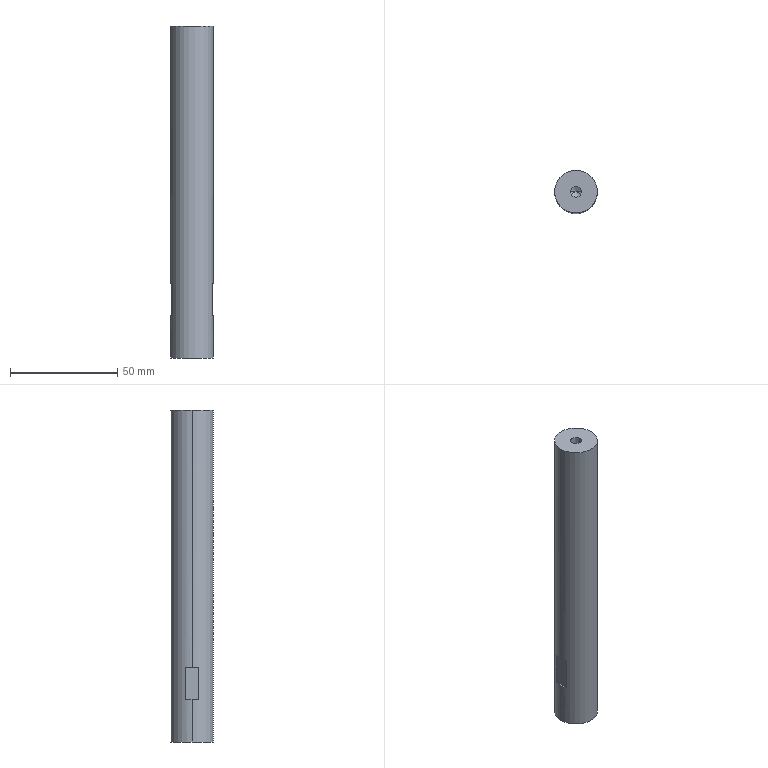Part | STEP file | slingshot displacement cylinder seat post | 1 solid | 18 faces | box 20 x 20 x 155 mm | volume 47945 mm3 | plane 8 | cylinder 6 | cone 4 | commonest cylinder face diameters 5 x4 20 x2
STEP:
#1=CARTESIAN_POINT('',(0.,0.,0.));
#2=DIRECTION('',(0.,0.,1.));
#3=DIRECTION('',(1.,0.,0.));
#4=AXIS2_PLACEMENT_3D('',#1,#2,#3);
#5=CARTESIAN_POINT('',(-2.5,0.,138.));
#6=VERTEX_POINT('',#5);
#7=CARTESIAN_POINT('',(2.5,0.,138.));
#8=VERTEX_POINT('',#7);
#9=CARTESIAN_POINT('',(0.,0.,138.));
#10=DIRECTION('',(0.,0.,1.));
#11=DIRECTION('',(1.,0.,0.));
#12=AXIS2_PLACEMENT_3D('',#9,#10,#11);
#13=CIRCLE('',#12,2.5);
#14=CARTESIAN_POINT('',(0.,0.,138.));
#15=DIRECTION('',(0.,0.,1.));
#16=DIRECTION('',(1.,0.,0.));
#17=AXIS2_PLACEMENT_3D('',#14,#15,#16);
#18=CONICAL_SURFACE('',#17,2.5,1.03);
#19=CARTESIAN_POINT('',(0.,0.));
#20=DIRECTION('',(1.,0.));
#21=VECTOR('',#20,1.);
#22=LINE('',#19,#21);
#23=(GEOMETRIC_REPRESENTATION_CONTEXT(2)PARAMETRIC_REPRESENTATION_CONTEXT()REPRESENTATION_CONTEXT('',''));
#24=DEFINITIONAL_REPRESENTATION('',(#22),#23);
#25=PCURVE('',#18,#24);
#26=CARTESIAN_POINT('',(0.,0.,155.));
#27=DIRECTION('',(0.,0.,1.));
#28=DIRECTION('',(1.,0.,0.));
#29=AXIS2_PLACEMENT_3D('',#26,#27,#28);
#30=CYLINDRICAL_SURFACE('',#29,2.5);
#31=CARTESIAN_POINT('',(0.,-17.));
#32=DIRECTION('',(1.,0.));
#33=VECTOR('',#32,1.);
#34=LINE('',#31,#33);
#35=(GEOMETRIC_REPRESENTATION_CONTEXT(2)PARAMETRIC_REPRESENTATION_CONTEXT()REPRESENTATION_CONTEXT('',''));
#36=DEFINITIONAL_REPRESENTATION('',(#34),#35);
#37=PCURVE('',#30,#36);
#38=SURFACE_CURVE('',#13,(#25,#37),.PCURVE_S1.);
#39=EDGE_CURVE('',#6,#8,#38,.T.);
#40=ORIENTED_EDGE('',*,*,#39,.F.);
#41=CARTESIAN_POINT('',(0.,0.,136.498));
#42=VERTEX_POINT('',#41);
#43=CARTESIAN_POINT('',(-2.5,0.,138.));
#44=DIRECTION('',(-0.8572,0.,0.515));
#45=VECTOR('',#44,1.);
#46=LINE('',#43,#45);
#47=CARTESIAN_POINT('',(3.142,0.));
#48=DIRECTION('',(0.,1.));
#49=VECTOR('',#48,1.);
#50=LINE('',#47,#49);
#51=(GEOMETRIC_REPRESENTATION_CONTEXT(2)PARAMETRIC_REPRESENTATION_CONTEXT()REPRESENTATION_CONTEXT('',''));
#52=DEFINITIONAL_REPRESENTATION('',(#50),#51);
#53=PCURVE('',#18,#52);
#54=CARTESIAN_POINT('',(0.,0.,138.));
#55=DIRECTION('',(0.,0.,1.));
#56=DIRECTION('',(1.,0.,0.));
#57=AXIS2_PLACEMENT_3D('',#54,#55,#56);
#58=CONICAL_SURFACE('',#57,2.5,1.03);
#59=CARTESIAN_POINT('',(3.142,0.));
#60=DIRECTION('',(0.,1.));
#61=VECTOR('',#60,1.);
#62=LINE('',#59,#61);
#63=(GEOMETRIC_REPRESENTATION_CONTEXT(2)PARAMETRIC_REPRESENTATION_CONTEXT()REPRESENTATION_CONTEXT('',''));
#64=DEFINITIONAL_REPRESENTATION('',(#62),#63);
#65=PCURVE('',#58,#64);
#66=SURFACE_CURVE('',#46,(#53,#65),.PCURVE_S1.);
#67=EDGE_CURVE('',#42,#6,#66,.T.);
#68=ORIENTED_EDGE('',*,*,#67,.F.);
#69=CARTESIAN_POINT('',(2.5,0.,138.));
#70=DIRECTION('',(0.8572,0.,0.515));
#71=VECTOR('',#70,1.);
#72=LINE('',#69,#71);
#73=CARTESIAN_POINT('',(6.283,0.));
#74=DIRECTION('',(0.,1.));
#75=VECTOR('',#74,1.);
#76=LINE('',#73,#75);
#77=(GEOMETRIC_REPRESENTATION_CONTEXT(2)PARAMETRIC_REPRESENTATION_CONTEXT()REPRESENTATION_CONTEXT('',''));
#78=DEFINITIONAL_REPRESENTATION('',(#76),#77);
#79=PCURVE('',#18,#78);
#80=CARTESIAN_POINT('',(0.,0.));
#81=DIRECTION('',(0.,1.));
#82=VECTOR('',#81,1.);
#83=LINE('',#80,#82);
#84=(GEOMETRIC_REPRESENTATION_CONTEXT(2)PARAMETRIC_REPRESENTATION_CONTEXT()REPRESENTATION_CONTEXT('',''));
#85=DEFINITIONAL_REPRESENTATION('',(#83),#84);
#86=PCURVE('',#58,#85);
#87=SURFACE_CURVE('',#72,(#79,#86),.PCURVE_S1.);
#88=EDGE_CURVE('',#42,#8,#87,.T.);
#89=ORIENTED_EDGE('',*,*,#88,.T.);
#90=EDGE_LOOP('',(#40,#68,#89));
#91=FACE_BOUND('',#90,.F.);
#92=ADVANCED_FACE('',(#91),#18,.F.);
#93=CARTESIAN_POINT('',(2.5,0.,155.));
#94=VERTEX_POINT('',#93);
#95=CARTESIAN_POINT('',(2.5,0.,155.));
#96=DIRECTION('',(0.,0.,1.));
#97=VECTOR('',#96,1.);
#98=LINE('',#95,#97);
#99=CARTESIAN_POINT('',(6.283,0.));
#100=DIRECTION('',(0.,1.));
#101=VECTOR('',#100,1.);
#102=LINE('',#99,#101);
#103=(GEOMETRIC_REPRESENTATION_CONTEXT(2)PARAMETRIC_REPRESENTATION_CONTEXT()REPRESENTATION_CONTEXT('',''));
#104=DEFINITIONAL_REPRESENTATION('',(#102),#103);
#105=PCURVE('',#30,#104);
#106=CARTESIAN_POINT('',(0.,0.,155.));
#107=DIRECTION('',(0.,0.,1.));
#108=DIRECTION('',(1.,0.,0.));
#109=AXIS2_PLACEMENT_3D('',#106,#107,#108);
#110=CYLINDRICAL_SURFACE('',#109,2.5);
#111=CARTESIAN_POINT('',(0.,0.));
#112=DIRECTION('',(0.,1.));
#113=VECTOR('',#112,1.);
#114=LINE('',#111,#113);
#115=(GEOMETRIC_REPRESENTATION_CONTEXT(2)PARAMETRIC_REPRESENTATION_CONTEXT()REPRESENTATION_CONTEXT('',''));
#116=DEFINITIONAL_REPRESENTATION('',(#114),#115);
#117=PCURVE('',#110,#116);
#118=SURFACE_CURVE('',#98,(#105,#117),.PCURVE_S1.);
#119=EDGE_CURVE('',#8,#94,#118,.T.);
#120=ORIENTED_EDGE('',*,*,#119,.T.);
#121=CARTESIAN_POINT('',(-2.5,0.,155.));
#122=VERTEX_POINT('',#121);
#123=CARTESIAN_POINT('',(0.,0.,155.));
#124=DIRECTION('',(0.,0.,1.));
#125=DIRECTION('',(1.,0.,0.));
#126=AXIS2_PLACEMENT_3D('',#123,#124,#125);
#127=CIRCLE('',#126,2.5);
#128=CARTESIAN_POINT('',(0.,0.));
#129=DIRECTION('',(1.,0.));
#130=VECTOR('',#129,1.);
#131=LINE('',#128,#130);
#132=(GEOMETRIC_REPRESENTATION_CONTEXT(2)PARAMETRIC_REPRESENTATION_CONTEXT()REPRESENTATION_CONTEXT('',''));
#133=DEFINITIONAL_REPRESENTATION('',(#131),#132);
#134=PCURVE('',#30,#133);
#135=CARTESIAN_POINT('',(0.,0.,155.));
#136=DIRECTION('',(0.,0.,1.));
#137=DIRECTION('',(1.,0.,0.));
#138=AXIS2_PLACEMENT_3D('',#135,#136,#137);
#139=PLANE('',#138);
#140=CARTESIAN_POINT('',(0.,0.));
#141=DIRECTION('',(1.,0.));
#142=AXIS2_PLACEMENT_2D('',#140,#141);
#143=CIRCLE('',#142,2.5);
#144=(GEOMETRIC_REPRESENTATION_CONTEXT(2)PARAMETRIC_REPRESENTATION_CONTEXT()REPRESENTATION_CONTEXT('',''));
#145=DEFINITIONAL_REPRESENTATION('',(#143),#144);
#146=PCURVE('',#139,#145);
#147=SURFACE_CURVE('',#127,(#134,#146),.PCURVE_S1.);
#148=EDGE_CURVE('',#122,#94,#147,.T.);
#149=ORIENTED_EDGE('',*,*,#148,.F.);
#150=CARTESIAN_POINT('',(-2.5,0.,155.));
#151=DIRECTION('',(0.,0.,1.));
#152=VECTOR('',#151,1.);
#153=LINE('',#150,#152);
#154=CARTESIAN_POINT('',(3.142,0.));
#155=DIRECTION('',(0.,1.));
#156=VECTOR('',#155,1.);
#157=LINE('',#154,#156);
#158=(GEOMETRIC_REPRESENTATION_CONTEXT(2)PARAMETRIC_REPRESENTATION_CONTEXT()REPRESENTATION_CONTEXT('',''));
#159=DEFINITIONAL_REPRESENTATION('',(#157),#158);
#160=PCURVE('',#30,#159);
#161=CARTESIAN_POINT('',(3.142,0.));
#162=DIRECTION('',(0.,1.));
#163=VECTOR('',#162,1.);
#164=LINE('',#161,#163);
#165=(GEOMETRIC_REPRESENTATION_CONTEXT(2)PARAMETRIC_REPRESENTATION_CONTEXT()REPRESENTATION_CONTEXT('',''));
#166=DEFINITIONAL_REPRESENTATION('',(#164),#165);
#167=PCURVE('',#110,#166);
#168=SURFACE_CURVE('',#153,(#160,#167),.PCURVE_S1.);
#169=EDGE_CURVE('',#6,#122,#168,.T.);
#170=ORIENTED_EDGE('',*,*,#169,.F.);
#171=ORIENTED_EDGE('',*,*,#39,.T.);
#172=EDGE_LOOP('',(#120,#149,#170,#171));
#173=FACE_BOUND('',#172,.F.);
#174=ADVANCED_FACE('',(#173),#30,.F.);
#175=CARTESIAN_POINT('',(2.5,0.,17.));
#176=VERTEX_POINT('',#175);
#177=CARTESIAN_POINT('',(-2.5,0.,17.));
#178=VERTEX_POINT('',#177);
#179=CARTESIAN_POINT('',(0.,0.,17.));
#180=DIRECTION('',(0.,0.,-1.));
#181=DIRECTION('',(-1.,0.,0.));
#182=AXIS2_PLACEMENT_3D('',#179,#180,#181);
#183=CIRCLE('',#182,2.5);
#184=CARTESIAN_POINT('',(0.,0.,17.));
#185=DIRECTION('',(0.,0.,-1.));
#186=DIRECTION('',(-1.,0.,0.));
#187=AXIS2_PLACEMENT_3D('',#184,#185,#186);
#188=CONICAL_SURFACE('',#187,2.5,1.03);
#189=CARTESIAN_POINT('',(0.,0.));
#190=DIRECTION('',(1.,0.));
#191=VECTOR('',#190,1.);
#192=LINE('',#189,#191);
#193=(GEOMETRIC_REPRESENTATION_CONTEXT(2)PARAMETRIC_REPRESENTATION_CONTEXT()REPRESENTATION_CONTEXT('',''));
#194=DEFINITIONAL_REPRESENTATION('',(#192),#193);
#195=PCURVE('',#188,#194);
#196=CARTESIAN_POINT('',(0.,0.,0.));
#197=DIRECTION('',(0.,0.,-1.));
#198=DIRECTION('',(-1.,0.,0.));
#199=AXIS2_PLACEMENT_3D('',#196,#197,#198);
#200=CYLINDRICAL_SURFACE('',#199,2.5);
#201=CARTESIAN_POINT('',(0.,-17.));
#202=DIRECTION('',(1.,0.));
#203=VECTOR('',#202,1.);
#204=LINE('',#201,#203);
#205=(GEOMETRIC_REPRESENTATION_CONTEXT(2)PARAMETRIC_REPRESENTATION_CONTEXT()REPRESENTATION_CONTEXT('',''));
#206=DEFINITIONAL_REPRESENTATION('',(#204),#205);
#207=PCURVE('',#200,#206);
#208=SURFACE_CURVE('',#183,(#195,#207),.PCURVE_S1.);
#209=EDGE_CURVE('',#176,#178,#208,.T.);
#210=ORIENTED_EDGE('',*,*,#209,.F.);
#211=CARTESIAN_POINT('',(0.,0.,18.502));
#212=VERTEX_POINT('',#211);
#213=CARTESIAN_POINT('',(2.5,0.,17.));
#214=DIRECTION('',(0.8572,0.,-0.515));
#215=VECTOR('',#214,1.);
#216=LINE('',#213,#215);
#217=CARTESIAN_POINT('',(3.142,0.));
#218=DIRECTION('',(0.,1.));
#219=VECTOR('',#218,1.);
#220=LINE('',#217,#219);
#221=(GEOMETRIC_REPRESENTATION_CONTEXT(2)PARAMETRIC_REPRESENTATION_CONTEXT()REPRESENTATION_CONTEXT('',''));
#222=DEFINITIONAL_REPRESENTATION('',(#220),#221);
#223=PCURVE('',#188,#222);
#224=CARTESIAN_POINT('',(0.,0.,17.));
#225=DIRECTION('',(0.,0.,-1.));
#226=DIRECTION('',(-1.,0.,0.));
#227=AXIS2_PLACEMENT_3D('',#224,#225,#226);
#228=CONICAL_SURFACE('',#227,2.5,1.03);
#229=CARTESIAN_POINT('',(3.142,0.));
#230=DIRECTION('',(0.,1.));
#231=VECTOR('',#230,1.);
#232=LINE('',#229,#231);
#233=(GEOMETRIC_REPRESENTATION_CONTEXT(2)PARAMETRIC_REPRESENTATION_CONTEXT()REPRESENTATION_CONTEXT('',''));
#234=DEFINITIONAL_REPRESENTATION('',(#232),#233);
#235=PCURVE('',#228,#234);
#236=SURFACE_CURVE('',#216,(#223,#235),.PCURVE_S1.);
#237=EDGE_CURVE('',#212,#176,#236,.T.);
#238=ORIENTED_EDGE('',*,*,#237,.F.);
#239=CARTESIAN_POINT('',(-2.5,0.,17.));
#240=DIRECTION('',(-0.8572,0.,-0.515));
#241=VECTOR('',#240,1.);
#242=LINE('',#239,#241);
#243=CARTESIAN_POINT('',(6.283,0.));
#244=DIRECTION('',(0.,1.));
#245=VECTOR('',#244,1.);
#246=LINE('',#243,#245);
#247=(GEOMETRIC_REPRESENTATION_CONTEXT(2)PARAMETRIC_REPRESENTATION_CONTEXT()REPRESENTATION_CONTEXT('',''));
#248=DEFINITIONAL_REPRESENTATION('',(#246),#247);
#249=PCURVE('',#188,#248);
#250=CARTESIAN_POINT('',(0.,0.));
#251=DIRECTION('',(0.,1.));
#252=VECTOR('',#251,1.);
#253=LINE('',#250,#252);
#254=(GEOMETRIC_REPRESENTATION_CONTEXT(2)PARAMETRIC_REPRESENTATION_CONTEXT()REPRESENTATION_CONTEXT('',''));
#255=DEFINITIONAL_REPRESENTATION('',(#253),#254);
#256=PCURVE('',#228,#255);
#257=SURFACE_CURVE('',#242,(#249,#256),.PCURVE_S1.);
#258=EDGE_CURVE('',#212,#178,#257,.T.);
#259=ORIENTED_EDGE('',*,*,#258,.T.);
#260=EDGE_LOOP('',(#210,#238,#259));
#261=FACE_BOUND('',#260,.F.);
#262=ADVANCED_FACE('',(#261),#188,.F.);
#263=CARTESIAN_POINT('',(-2.5,0.,0.));
#264=VERTEX_POINT('',#263);
#265=CARTESIAN_POINT('',(-2.5,0.,0.));
#266=DIRECTION('',(0.,0.,-1.));
#267=VECTOR('',#266,1.);
#268=LINE('',#265,#267);
#269=CARTESIAN_POINT('',(6.283,0.));
#270=DIRECTION('',(0.,1.));
#271=VECTOR('',#270,1.);
#272=LINE('',#269,#271);
#273=(GEOMETRIC_REPRESENTATION_CONTEXT(2)PARAMETRIC_REPRESENTATION_CONTEXT()REPRESENTATION_CONTEXT('',''));
#274=DEFINITIONAL_REPRESENTATION('',(#272),#273);
#275=PCURVE('',#200,#274);
#276=CARTESIAN_POINT('',(0.,0.,0.));
#277=DIRECTION('',(0.,0.,-1.));
#278=DIRECTION('',(-1.,0.,0.));
#279=AXIS2_PLACEMENT_3D('',#276,#277,#278);
#280=CYLINDRICAL_SURFACE('',#279,2.5);
#281=CARTESIAN_POINT('',(0.,0.));
#282=DIRECTION('',(0.,1.));
#283=VECTOR('',#282,1.);
#284=LINE('',#281,#283);
#285=(GEOMETRIC_REPRESENTATION_CONTEXT(2)PARAMETRIC_REPRESENTATION_CONTEXT()REPRESENTATION_CONTEXT('',''));
#286=DEFINITIONAL_REPRESENTATION('',(#284),#285);
#287=PCURVE('',#280,#286);
#288=SURFACE_CURVE('',#268,(#275,#287),.PCURVE_S1.);
#289=EDGE_CURVE('',#178,#264,#288,.T.);
#290=ORIENTED_EDGE('',*,*,#289,.T.);
#291=CARTESIAN_POINT('',(2.5,0.,0.));
#292=VERTEX_POINT('',#291);
#293=CARTESIAN_POINT('',(0.,0.,0.));
#294=DIRECTION('',(0.,0.,-1.));
#295=DIRECTION('',(-1.,0.,0.));
#296=AXIS2_PLACEMENT_3D('',#293,#294,#295);
#297=CIRCLE('',#296,2.5);
#298=CARTESIAN_POINT('',(0.,0.));
#299=DIRECTION('',(1.,0.));
#300=VECTOR('',#299,1.);
#301=LINE('',#298,#300);
#302=(GEOMETRIC_REPRESENTATION_CONTEXT(2)PARAMETRIC_REPRESENTATION_CONTEXT()REPRESENTATION_CONTEXT('',''));
#303=DEFINITIONAL_REPRESENTATION('',(#301),#302);
#304=PCURVE('',#200,#303);
#305=CARTESIAN_POINT('',(0.,0.,0.));
#306=DIRECTION('',(0.,0.,1.));
#307=DIRECTION('',(1.,0.,0.));
#308=AXIS2_PLACEMENT_3D('',#305,#306,#307);
#309=PLANE('',#308);
#310=CARTESIAN_POINT('',(-2.5,0.));
#311=CARTESIAN_POINT('',(-2.5,4.33));
#312=CARTESIAN_POINT('',(1.25,2.165));
#313=CARTESIAN_POINT('',(5.,0.));
#314=CARTESIAN_POINT('',(1.25,-2.165));
#315=CARTESIAN_POINT('',(-2.5,-4.33));
#316=CARTESIAN_POINT('',(-2.5,0.));
#317=(BOUNDED_CURVE()B_SPLINE_CURVE(2,(#310,#311,#312,#313,#314,#315,#316),.UNSPECIFIED.,.T.,.F.)B_SPLINE_CURVE_WITH_KNOTS((1,2,2,2,2,1),(-2.094,0.,2.094,4.189,6.283,8.378),.UNSPECIFIED.)CURVE()GEOMETRIC_REPRESENTATION_ITEM()RATIONAL_B_SPLINE_CURVE((1.,0.5,1.,0.5,1.,0.5,1.))REPRESENTATION_ITEM(''));
#318=(GEOMETRIC_REPRESENTATION_CONTEXT(2)PARAMETRIC_REPRESENTATION_CONTEXT()REPRESENTATION_CONTEXT('',''));
#319=DEFINITIONAL_REPRESENTATION('',(#317),#318);
#320=PCURVE('',#309,#319);
#321=SURFACE_CURVE('',#297,(#304,#320),.PCURVE_S1.);
#322=EDGE_CURVE('',#292,#264,#321,.T.);
#323=ORIENTED_EDGE('',*,*,#322,.F.);
#324=CARTESIAN_POINT('',(2.5,0.,0.));
#325=DIRECTION('',(0.,0.,-1.));
#326=VECTOR('',#325,1.);
#327=LINE('',#324,#326);
#328=CARTESIAN_POINT('',(3.142,0.));
#329=DIRECTION('',(0.,1.));
#330=VECTOR('',#329,1.);
#331=LINE('',#328,#330);
#332=(GEOMETRIC_REPRESENTATION_CONTEXT(2)PARAMETRIC_REPRESENTATION_CONTEXT()REPRESENTATION_CONTEXT('',''));
#333=DEFINITIONAL_REPRESENTATION('',(#331),#332);
#334=PCURVE('',#200,#333);
#335=CARTESIAN_POINT('',(3.142,0.));
#336=DIRECTION('',(0.,1.));
#337=VECTOR('',#336,1.);
#338=LINE('',#335,#337);
#339=(GEOMETRIC_REPRESENTATION_CONTEXT(2)PARAMETRIC_REPRESENTATION_CONTEXT()REPRESENTATION_CONTEXT('',''));
#340=DEFINITIONAL_REPRESENTATION('',(#338),#339);
#341=PCURVE('',#280,#340);
#342=SURFACE_CURVE('',#327,(#334,#341),.PCURVE_S1.);
#343=EDGE_CURVE('',#176,#292,#342,.T.);
#344=ORIENTED_EDGE('',*,*,#343,.F.);
#345=ORIENTED_EDGE('',*,*,#209,.T.);
#346=EDGE_LOOP('',(#290,#323,#344,#345));
#347=FACE_BOUND('',#346,.F.);
#348=ADVANCED_FACE('',(#347),#200,.F.);
#349=CARTESIAN_POINT('',(10.,0.,155.));
#350=VERTEX_POINT('',#349);
#351=CARTESIAN_POINT('',(-10.,0.,155.));
#352=VERTEX_POINT('',#351);
#353=CARTESIAN_POINT('',(0.,0.,155.));
#354=DIRECTION('',(0.,0.,1.));
#355=DIRECTION('',(1.,0.,0.));
#356=AXIS2_PLACEMENT_3D('',#353,#354,#355);
#357=CIRCLE('',#356,10.);
#358=CARTESIAN_POINT('',(0.,0.,155.));
#359=DIRECTION('',(0.,0.,-1.));
#360=DIRECTION('',(-1.,0.,0.));
#361=AXIS2_PLACEMENT_3D('',#358,#359,#360);
#362=CYLINDRICAL_SURFACE('',#361,10.);
#363=CARTESIAN_POINT('',(3.142,0.));
#364=DIRECTION('',(-1.,0.));
#365=VECTOR('',#364,1.);
#366=LINE('',#363,#365);
#367=(GEOMETRIC_REPRESENTATION_CONTEXT(2)PARAMETRIC_REPRESENTATION_CONTEXT()REPRESENTATION_CONTEXT('',''));
#368=DEFINITIONAL_REPRESENTATION('',(#366),#367);
#369=PCURVE('',#362,#368);
#370=CARTESIAN_POINT('',(0.,0.));
#371=DIRECTION('',(1.,0.));
#372=AXIS2_PLACEMENT_2D('',#370,#371);
#373=CIRCLE('',#372,10.);
#374=(GEOMETRIC_REPRESENTATION_CONTEXT(2)PARAMETRIC_REPRESENTATION_CONTEXT()REPRESENTATION_CONTEXT('',''));
#375=DEFINITIONAL_REPRESENTATION('',(#373),#374);
#376=PCURVE('',#139,#375);
#377=SURFACE_CURVE('',#357,(#369,#376),.PCURVE_S1.);
#378=EDGE_CURVE('',#350,#352,#377,.T.);
#379=ORIENTED_EDGE('',*,*,#378,.F.);
#380=CARTESIAN_POINT('',(10.,0.,35.));
#381=VERTEX_POINT('',#380);
#382=CARTESIAN_POINT('',(10.,0.,155.));
#383=DIRECTION('',(0.,0.,-1.));
#384=VECTOR('',#383,1.);
#385=LINE('',#382,#384);
#386=CARTESIAN_POINT('',(3.142,0.));
#387=DIRECTION('',(0.,1.));
#388=VECTOR('',#387,1.);
#389=LINE('',#386,#388);
#390=(GEOMETRIC_REPRESENTATION_CONTEXT(2)PARAMETRIC_REPRESENTATION_CONTEXT()REPRESENTATION_CONTEXT('',''));
#391=DEFINITIONAL_REPRESENTATION('',(#389),#390);
#392=PCURVE('',#362,#391);
#393=CARTESIAN_POINT('',(0.,0.,155.));
#394=DIRECTION('',(0.,0.,-1.));
#395=DIRECTION('',(-1.,0.,0.));
#396=AXIS2_PLACEMENT_3D('',#393,#394,#395);
#397=CYLINDRICAL_SURFACE('',#396,10.);
#398=CARTESIAN_POINT('',(3.142,0.));
#399=DIRECTION('',(0.,1.));
#400=VECTOR('',#399,1.);
#401=LINE('',#398,#400);
#402=(GEOMETRIC_REPRESENTATION_CONTEXT(2)PARAMETRIC_REPRESENTATION_CONTEXT()REPRESENTATION_CONTEXT('',''));
#403=DEFINITIONAL_REPRESENTATION('',(#401),#402);
#404=PCURVE('',#397,#403);
#405=SURFACE_CURVE('',#385,(#392,#404),.PCURVE_S1.);
#406=EDGE_CURVE('',#350,#381,#405,.T.);
#407=ORIENTED_EDGE('',*,*,#406,.T.);
#408=CARTESIAN_POINT('',(9.5,3.122,35.));
#409=VERTEX_POINT('',#408);
#410=CARTESIAN_POINT('',(0.,0.,35.));
#411=DIRECTION('',(0.,0.,-1.));
#412=DIRECTION('',(-1.,0.,0.));
#413=AXIS2_PLACEMENT_3D('',#410,#411,#412);
#414=CIRCLE('',#413,10.);
#415=CARTESIAN_POINT('',(0.,120.));
#416=DIRECTION('',(1.,0.));
#417=VECTOR('',#416,1.);
#418=LINE('',#415,#417);
#419=(GEOMETRIC_REPRESENTATION_CONTEXT(2)PARAMETRIC_REPRESENTATION_CONTEXT()REPRESENTATION_CONTEXT('',''));
#420=DEFINITIONAL_REPRESENTATION('',(#418),#419);
#421=PCURVE('',#362,#420);
#422=CARTESIAN_POINT('',(30.33,174.5,35.));
#423=DIRECTION('',(0.,0.,-1.));
#424=DIRECTION('',(-1.,0.,0.));
#425=AXIS2_PLACEMENT_3D('',#422,#423,#424);
#426=PLANE('',#425);
#427=CARTESIAN_POINT('',(30.33,-174.5));
#428=DIRECTION('',(1.,0.));
#429=AXIS2_PLACEMENT_2D('',#427,#428);
#430=CIRCLE('',#429,10.);
#431=(GEOMETRIC_REPRESENTATION_CONTEXT(2)PARAMETRIC_REPRESENTATION_CONTEXT()REPRESENTATION_CONTEXT('',''));
#432=DEFINITIONAL_REPRESENTATION('',(#430),#431);
#433=PCURVE('',#426,#432);
#434=SURFACE_CURVE('',#414,(#421,#433),.PCURVE_S1.);
#435=EDGE_CURVE('',#409,#381,#434,.T.);
#436=ORIENTED_EDGE('',*,*,#435,.F.);
#437=CARTESIAN_POINT('',(9.5,3.122,20.));
#438=VERTEX_POINT('',#437);
#439=CARTESIAN_POINT('',(9.5,3.122,155.));
#440=DIRECTION('',(0.,0.,1.));
#441=VECTOR('',#440,1.);
#442=LINE('',#439,#441);
#443=CARTESIAN_POINT('',(2.824,0.));
#444=DIRECTION('',(0.,-1.));
#445=VECTOR('',#444,1.);
#446=LINE('',#443,#445);
#447=(GEOMETRIC_REPRESENTATION_CONTEXT(2)PARAMETRIC_REPRESENTATION_CONTEXT()REPRESENTATION_CONTEXT('',''));
#448=DEFINITIONAL_REPRESENTATION('',(#446),#447);
#449=PCURVE('',#362,#448);
#450=CARTESIAN_POINT('',(9.5,174.5,20.));
#451=DIRECTION('',(1.,0.,0.));
#452=DIRECTION('',(0.,0.,-1.));
#453=AXIS2_PLACEMENT_3D('',#450,#451,#452);
#454=PLANE('',#453);
#455=CARTESIAN_POINT('',(-135.,-171.378));
#456=DIRECTION('',(-1.,0.));
#457=VECTOR('',#456,1.);
#458=LINE('',#455,#457);
#459=(GEOMETRIC_REPRESENTATION_CONTEXT(2)PARAMETRIC_REPRESENTATION_CONTEXT()REPRESENTATION_CONTEXT('',''));
#460=DEFINITIONAL_REPRESENTATION('',(#458),#459);
#461=PCURVE('',#454,#460);
#462=SURFACE_CURVE('',#442,(#449,#461),.PCURVE_S1.);
#463=EDGE_CURVE('',#438,#409,#462,.T.);
#464=ORIENTED_EDGE('',*,*,#463,.F.);
#465=CARTESIAN_POINT('',(10.,0.,20.));
#466=VERTEX_POINT('',#465);
#467=CARTESIAN_POINT('',(0.,0.,20.));
#468=DIRECTION('',(0.,0.,1.));
#469=DIRECTION('',(1.,0.,0.));
#470=AXIS2_PLACEMENT_3D('',#467,#468,#469);
#471=CIRCLE('',#470,10.);
#472=CARTESIAN_POINT('',(3.142,135.));
#473=DIRECTION('',(-1.,0.));
#474=VECTOR('',#473,1.);
#475=LINE('',#472,#474);
#476=(GEOMETRIC_REPRESENTATION_CONTEXT(2)PARAMETRIC_REPRESENTATION_CONTEXT()REPRESENTATION_CONTEXT('',''));
#477=DEFINITIONAL_REPRESENTATION('',(#475),#476);
#478=PCURVE('',#362,#477);
#479=CARTESIAN_POINT('',(30.33,174.5,20.));
#480=DIRECTION('',(0.,0.,1.));
#481=DIRECTION('',(1.,0.,0.));
#482=AXIS2_PLACEMENT_3D('',#479,#480,#481);
#483=PLANE('',#482);
#484=CARTESIAN_POINT('',(-30.33,-174.5));
#485=DIRECTION('',(1.,0.));
#486=AXIS2_PLACEMENT_2D('',#484,#485);
#487=CIRCLE('',#486,10.);
#488=(GEOMETRIC_REPRESENTATION_CONTEXT(2)PARAMETRIC_REPRESENTATION_CONTEXT()REPRESENTATION_CONTEXT('',''));
#489=DEFINITIONAL_REPRESENTATION('',(#487),#488);
#490=PCURVE('',#483,#489);
#491=SURFACE_CURVE('',#471,(#478,#490),.PCURVE_S1.);
#492=EDGE_CURVE('',#466,#438,#491,.T.);
#493=ORIENTED_EDGE('',*,*,#492,.F.);
#494=CARTESIAN_POINT('',(10.,0.,0.));
#495=VERTEX_POINT('',#494);
#496=CARTESIAN_POINT('',(10.,0.,155.));
#497=DIRECTION('',(0.,0.,-1.));
#498=VECTOR('',#497,1.);
#499=LINE('',#496,#498);
#500=CARTESIAN_POINT('',(3.142,0.));
#501=DIRECTION('',(0.,1.));
#502=VECTOR('',#501,1.);
#503=LINE('',#500,#502);
#504=(GEOMETRIC_REPRESENTATION_CONTEXT(2)PARAMETRIC_REPRESENTATION_CONTEXT()REPRESENTATION_CONTEXT('',''));
#505=DEFINITIONAL_REPRESENTATION('',(#503),#504);
#506=PCURVE('',#362,#505);
#507=CARTESIAN_POINT('',(3.142,0.));
#508=DIRECTION('',(0.,1.));
#509=VECTOR('',#508,1.);
#510=LINE('',#507,#509);
#511=(GEOMETRIC_REPRESENTATION_CONTEXT(2)PARAMETRIC_REPRESENTATION_CONTEXT()REPRESENTATION_CONTEXT('',''));
#512=DEFINITIONAL_REPRESENTATION('',(#510),#511);
#513=PCURVE('',#397,#512);
#514=SURFACE_CURVE('',#499,(#506,#513),.PCURVE_S1.);
#515=EDGE_CURVE('',#466,#495,#514,.T.);
#516=ORIENTED_EDGE('',*,*,#515,.T.);
#517=CARTESIAN_POINT('',(-10.,0.,0.));
#518=VERTEX_POINT('',#517);
#519=CARTESIAN_POINT('',(0.,0.,0.));
#520=DIRECTION('',(0.,0.,1.));
#521=DIRECTION('',(1.,0.,0.));
#522=AXIS2_PLACEMENT_3D('',#519,#520,#521);
#523=CIRCLE('',#522,10.);
#524=CARTESIAN_POINT('',(3.142,155.));
#525=DIRECTION('',(-1.,0.));
#526=VECTOR('',#525,1.);
#527=LINE('',#524,#526);
#528=(GEOMETRIC_REPRESENTATION_CONTEXT(2)PARAMETRIC_REPRESENTATION_CONTEXT()REPRESENTATION_CONTEXT('',''));
#529=DEFINITIONAL_REPRESENTATION('',(#527),#528);
#530=PCURVE('',#362,#529);
#531=CARTESIAN_POINT('',(0.,0.));
#532=DIRECTION('',(1.,0.));
#533=AXIS2_PLACEMENT_2D('',#531,#532);
#534=CIRCLE('',#533,10.);
#535=(GEOMETRIC_REPRESENTATION_CONTEXT(2)PARAMETRIC_REPRESENTATION_CONTEXT()REPRESENTATION_CONTEXT('',''));
#536=DEFINITIONAL_REPRESENTATION('',(#534),#535);
#537=PCURVE('',#309,#536);
#538=SURFACE_CURVE('',#523,(#530,#537),.PCURVE_S1.);
#539=EDGE_CURVE('',#495,#518,#538,.T.);
#540=ORIENTED_EDGE('',*,*,#539,.T.);
#541=CARTESIAN_POINT('',(-10.,0.,20.));
#542=VERTEX_POINT('',#541);
#543=CARTESIAN_POINT('',(-10.,0.,155.));
#544=DIRECTION('',(0.,0.,-1.));
#545=VECTOR('',#544,1.);
#546=LINE('',#543,#545);
#547=CARTESIAN_POINT('',(0.,0.));
#548=DIRECTION('',(0.,1.));
#549=VECTOR('',#548,1.);
#550=LINE('',#547,#549);
#551=(GEOMETRIC_REPRESENTATION_CONTEXT(2)PARAMETRIC_REPRESENTATION_CONTEXT()REPRESENTATION_CONTEXT('',''));
#552=DEFINITIONAL_REPRESENTATION('',(#550),#551);
#553=PCURVE('',#362,#552);
#554=CARTESIAN_POINT('',(6.283,0.));
#555=DIRECTION('',(0.,1.));
#556=VECTOR('',#555,1.);
#557=LINE('',#554,#556);
#558=(GEOMETRIC_REPRESENTATION_CONTEXT(2)PARAMETRIC_REPRESENTATION_CONTEXT()REPRESENTATION_CONTEXT('',''));
#559=DEFINITIONAL_REPRESENTATION('',(#557),#558);
#560=PCURVE('',#397,#559);
#561=SURFACE_CURVE('',#546,(#553,#560),.PCURVE_S1.);
#562=EDGE_CURVE('',#542,#518,#561,.T.);
#563=ORIENTED_EDGE('',*,*,#562,.F.);
#564=CARTESIAN_POINT('',(-9.5,3.122,20.));
#565=VERTEX_POINT('',#564);
#566=CARTESIAN_POINT('',(0.,0.,20.));
#567=DIRECTION('',(0.,0.,1.));
#568=DIRECTION('',(1.,0.,0.));
#569=AXIS2_PLACEMENT_3D('',#566,#567,#568);
#570=CIRCLE('',#569,10.);
#571=CARTESIAN_POINT('',(3.142,135.));
#572=DIRECTION('',(-1.,0.));
#573=VECTOR('',#572,1.);
#574=LINE('',#571,#573);
#575=(GEOMETRIC_REPRESENTATION_CONTEXT(2)PARAMETRIC_REPRESENTATION_CONTEXT()REPRESENTATION_CONTEXT('',''));
#576=DEFINITIONAL_REPRESENTATION('',(#574),#575);
#577=PCURVE('',#362,#576);
#578=CARTESIAN_POINT('',(-23.737,174.5,20.));
#579=DIRECTION('',(0.,0.,1.));
#580=DIRECTION('',(1.,0.,0.));
#581=AXIS2_PLACEMENT_3D('',#578,#579,#580);
#582=PLANE('',#581);
#583=CARTESIAN_POINT('',(23.737,-174.5));
#584=DIRECTION('',(1.,0.));
#585=AXIS2_PLACEMENT_2D('',#583,#584);
#586=CIRCLE('',#585,10.);
#587=(GEOMETRIC_REPRESENTATION_CONTEXT(2)PARAMETRIC_REPRESENTATION_CONTEXT()REPRESENTATION_CONTEXT('',''));
#588=DEFINITIONAL_REPRESENTATION('',(#586),#587);
#589=PCURVE('',#582,#588);
#590=SURFACE_CURVE('',#570,(#577,#589),.PCURVE_S1.);
#591=EDGE_CURVE('',#565,#542,#590,.T.);
#592=ORIENTED_EDGE('',*,*,#591,.F.);
#593=CARTESIAN_POINT('',(-9.5,3.122,35.));
#594=VERTEX_POINT('',#593);
#595=CARTESIAN_POINT('',(-9.5,3.122,155.));
#596=DIRECTION('',(0.,0.,-1.));
#597=VECTOR('',#596,1.);
#598=LINE('',#595,#597);
#599=CARTESIAN_POINT('',(0.3176,0.));
#600=DIRECTION('',(0.,1.));
#601=VECTOR('',#600,1.);
#602=LINE('',#599,#601);
#603=(GEOMETRIC_REPRESENTATION_CONTEXT(2)PARAMETRIC_REPRESENTATION_CONTEXT()REPRESENTATION_CONTEXT('',''));
#604=DEFINITIONAL_REPRESENTATION('',(#602),#603);
#605=PCURVE('',#362,#604);
#606=CARTESIAN_POINT('',(-9.5,174.5,20.));
#607=DIRECTION('',(-1.,0.,0.));
#608=DIRECTION('',(0.,0.,1.));
#609=AXIS2_PLACEMENT_3D('',#606,#607,#608);
#610=PLANE('',#609);
#611=CARTESIAN_POINT('',(135.,-171.378));
#612=DIRECTION('',(-1.,0.));
#613=VECTOR('',#612,1.);
#614=LINE('',#611,#613);
#615=(GEOMETRIC_REPRESENTATION_CONTEXT(2)PARAMETRIC_REPRESENTATION_CONTEXT()REPRESENTATION_CONTEXT('',''));
#616=DEFINITIONAL_REPRESENTATION('',(#614),#615);
#617=PCURVE('',#610,#616);
#618=SURFACE_CURVE('',#598,(#605,#617),.PCURVE_S1.);
#619=EDGE_CURVE('',#594,#565,#618,.T.);
#620=ORIENTED_EDGE('',*,*,#619,.F.);
#621=CARTESIAN_POINT('',(-10.,0.,35.));
#622=VERTEX_POINT('',#621);
#623=CARTESIAN_POINT('',(0.,0.,35.));
#624=DIRECTION('',(0.,0.,-1.));
#625=DIRECTION('',(-1.,0.,0.));
#626=AXIS2_PLACEMENT_3D('',#623,#624,#625);
#627=CIRCLE('',#626,10.);
#628=CARTESIAN_POINT('',(0.,120.));
#629=DIRECTION('',(1.,0.));
#630=VECTOR('',#629,1.);
#631=LINE('',#628,#630);
#632=(GEOMETRIC_REPRESENTATION_CONTEXT(2)PARAMETRIC_REPRESENTATION_CONTEXT()REPRESENTATION_CONTEXT('',''));
#633=DEFINITIONAL_REPRESENTATION('',(#631),#632);
#634=PCURVE('',#362,#633);
#635=CARTESIAN_POINT('',(-23.737,174.5,35.));
#636=DIRECTION('',(0.,0.,-1.));
#637=DIRECTION('',(-1.,0.,0.));
#638=AXIS2_PLACEMENT_3D('',#635,#636,#637);
#639=PLANE('',#638);
#640=CARTESIAN_POINT('',(-23.737,-174.5));
#641=DIRECTION('',(1.,0.));
#642=AXIS2_PLACEMENT_2D('',#640,#641);
#643=CIRCLE('',#642,10.);
#644=(GEOMETRIC_REPRESENTATION_CONTEXT(2)PARAMETRIC_REPRESENTATION_CONTEXT()REPRESENTATION_CONTEXT('',''));
#645=DEFINITIONAL_REPRESENTATION('',(#643),#644);
#646=PCURVE('',#639,#645);
#647=SURFACE_CURVE('',#627,(#634,#646),.PCURVE_S1.);
#648=EDGE_CURVE('',#622,#594,#647,.T.);
#649=ORIENTED_EDGE('',*,*,#648,.F.);
#650=CARTESIAN_POINT('',(-10.,0.,155.));
#651=DIRECTION('',(0.,0.,-1.));
#652=VECTOR('',#651,1.);
#653=LINE('',#650,#652);
#654=CARTESIAN_POINT('',(0.,0.));
#655=DIRECTION('',(0.,1.));
#656=VECTOR('',#655,1.);
#657=LINE('',#654,#656);
#658=(GEOMETRIC_REPRESENTATION_CONTEXT(2)PARAMETRIC_REPRESENTATION_CONTEXT()REPRESENTATION_CONTEXT('',''));
#659=DEFINITIONAL_REPRESENTATION('',(#657),#658);
#660=PCURVE('',#362,#659);
#661=CARTESIAN_POINT('',(6.283,0.));
#662=DIRECTION('',(0.,1.));
#663=VECTOR('',#662,1.);
#664=LINE('',#661,#663);
#665=(GEOMETRIC_REPRESENTATION_CONTEXT(2)PARAMETRIC_REPRESENTATION_CONTEXT()REPRESENTATION_CONTEXT('',''));
#666=DEFINITIONAL_REPRESENTATION('',(#664),#665);
#667=PCURVE('',#397,#666);
#668=SURFACE_CURVE('',#653,(#660,#667),.PCURVE_S1.);
#669=EDGE_CURVE('',#352,#622,#668,.T.);
#670=ORIENTED_EDGE('',*,*,#669,.F.);
#671=EDGE_LOOP('',(#379,#407,#436,#464,#493,#516,#540,#563,#592,#620,#649,#670));
#672=FACE_BOUND('',#671,.T.);
#673=ADVANCED_FACE('',(#672),#362,.T.);
#674=ORIENTED_EDGE('',*,*,#406,.F.);
#675=CARTESIAN_POINT('',(0.,0.,155.));
#676=DIRECTION('',(0.,0.,1.));
#677=DIRECTION('',(1.,0.,0.));
#678=AXIS2_PLACEMENT_3D('',#675,#676,#677);
#679=CIRCLE('',#678,10.);
#680=CARTESIAN_POINT('',(9.425,0.));
#681=DIRECTION('',(-1.,0.));
#682=VECTOR('',#681,1.);
#683=LINE('',#680,#682);
#684=(GEOMETRIC_REPRESENTATION_CONTEXT(2)PARAMETRIC_REPRESENTATION_CONTEXT()REPRESENTATION_CONTEXT('',''));
#685=DEFINITIONAL_REPRESENTATION('',(#683),#684);
#686=PCURVE('',#397,#685);
#687=CARTESIAN_POINT('',(0.,0.));
#688=DIRECTION('',(1.,0.));
#689=AXIS2_PLACEMENT_2D('',#687,#688);
#690=CIRCLE('',#689,10.);
#691=(GEOMETRIC_REPRESENTATION_CONTEXT(2)PARAMETRIC_REPRESENTATION_CONTEXT()REPRESENTATION_CONTEXT('',''));
#692=DEFINITIONAL_REPRESENTATION('',(#690),#691);
#693=PCURVE('',#139,#692);
#694=SURFACE_CURVE('',#679,(#686,#693),.PCURVE_S1.);
#695=EDGE_CURVE('',#352,#350,#694,.T.);
#696=ORIENTED_EDGE('',*,*,#695,.F.);
#697=ORIENTED_EDGE('',*,*,#669,.T.);
#698=CARTESIAN_POINT('',(-9.5,-3.122,35.));
#699=VERTEX_POINT('',#698);
#700=CARTESIAN_POINT('',(0.,0.,35.));
#701=DIRECTION('',(0.,0.,-1.));
#702=DIRECTION('',(-1.,0.,0.));
#703=AXIS2_PLACEMENT_3D('',#700,#701,#702);
#704=CIRCLE('',#703,10.);
#705=CARTESIAN_POINT('',(0.,120.));
#706=DIRECTION('',(1.,0.));
#707=VECTOR('',#706,1.);
#708=LINE('',#705,#707);
#709=(GEOMETRIC_REPRESENTATION_CONTEXT(2)PARAMETRIC_REPRESENTATION_CONTEXT()REPRESENTATION_CONTEXT('',''));
#710=DEFINITIONAL_REPRESENTATION('',(#708),#709);
#711=PCURVE('',#397,#710);
#712=CARTESIAN_POINT('',(-23.737,-174.5));
#713=DIRECTION('',(1.,0.));
#714=AXIS2_PLACEMENT_2D('',#712,#713);
#715=CIRCLE('',#714,10.);
#716=(GEOMETRIC_REPRESENTATION_CONTEXT(2)PARAMETRIC_REPRESENTATION_CONTEXT()REPRESENTATION_CONTEXT('',''));
#717=DEFINITIONAL_REPRESENTATION('',(#715),#716);
#718=PCURVE('',#639,#717);
#719=SURFACE_CURVE('',#704,(#711,#718),.PCURVE_S1.);
#720=EDGE_CURVE('',#699,#622,#719,.T.);
#721=ORIENTED_EDGE('',*,*,#720,.F.);
#722=CARTESIAN_POINT('',(-9.5,-3.122,20.));
#723=VERTEX_POINT('',#722);
#724=CARTESIAN_POINT('',(-9.5,-3.122,155.));
#725=DIRECTION('',(0.,0.,1.));
#726=VECTOR('',#725,1.);
#727=LINE('',#724,#726);
#728=CARTESIAN_POINT('',(5.966,0.));
#729=DIRECTION('',(0.,-1.));
#730=VECTOR('',#729,1.);
#731=LINE('',#728,#730);
#732=(GEOMETRIC_REPRESENTATION_CONTEXT(2)PARAMETRIC_REPRESENTATION_CONTEXT()REPRESENTATION_CONTEXT('',''));
#733=DEFINITIONAL_REPRESENTATION('',(#731),#732);
#734=PCURVE('',#397,#733);
#735=CARTESIAN_POINT('',(135.,-177.622));
#736=DIRECTION('',(1.,0.));
#737=VECTOR('',#736,1.);
#738=LINE('',#735,#737);
#739=(GEOMETRIC_REPRESENTATION_CONTEXT(2)PARAMETRIC_REPRESENTATION_CONTEXT()REPRESENTATION_CONTEXT('',''));
#740=DEFINITIONAL_REPRESENTATION('',(#738),#739);
#741=PCURVE('',#610,#740);
#742=SURFACE_CURVE('',#727,(#734,#741),.PCURVE_S1.);
#743=EDGE_CURVE('',#723,#699,#742,.T.);
#744=ORIENTED_EDGE('',*,*,#743,.F.);
#745=CARTESIAN_POINT('',(0.,0.,20.));
#746=DIRECTION('',(0.,0.,1.));
#747=DIRECTION('',(1.,0.,0.));
#748=AXIS2_PLACEMENT_3D('',#745,#746,#747);
#749=CIRCLE('',#748,10.);
#750=CARTESIAN_POINT('',(9.425,135.));
#751=DIRECTION('',(-1.,0.));
#752=VECTOR('',#751,1.);
#753=LINE('',#750,#752);
#754=(GEOMETRIC_REPRESENTATION_CONTEXT(2)PARAMETRIC_REPRESENTATION_CONTEXT()REPRESENTATION_CONTEXT('',''));
#755=DEFINITIONAL_REPRESENTATION('',(#753),#754);
#756=PCURVE('',#397,#755);
#757=CARTESIAN_POINT('',(23.737,-174.5));
#758=DIRECTION('',(1.,0.));
#759=AXIS2_PLACEMENT_2D('',#757,#758);
#760=CIRCLE('',#759,10.);
#761=(GEOMETRIC_REPRESENTATION_CONTEXT(2)PARAMETRIC_REPRESENTATION_CONTEXT()REPRESENTATION_CONTEXT('',''));
#762=DEFINITIONAL_REPRESENTATION('',(#760),#761);
#763=PCURVE('',#582,#762);
#764=SURFACE_CURVE('',#749,(#756,#763),.PCURVE_S1.);
#765=EDGE_CURVE('',#542,#723,#764,.T.);
#766=ORIENTED_EDGE('',*,*,#765,.F.);
#767=ORIENTED_EDGE('',*,*,#562,.T.);
#768=CARTESIAN_POINT('',(0.,0.,0.));
#769=DIRECTION('',(0.,0.,1.));
#770=DIRECTION('',(1.,0.,0.));
#771=AXIS2_PLACEMENT_3D('',#768,#769,#770);
#772=CIRCLE('',#771,10.);
#773=CARTESIAN_POINT('',(9.425,155.));
#774=DIRECTION('',(-1.,0.));
#775=VECTOR('',#774,1.);
#776=LINE('',#773,#775);
#777=(GEOMETRIC_REPRESENTATION_CONTEXT(2)PARAMETRIC_REPRESENTATION_CONTEXT()REPRESENTATION_CONTEXT('',''));
#778=DEFINITIONAL_REPRESENTATION('',(#776),#777);
#779=PCURVE('',#397,#778);
#780=CARTESIAN_POINT('',(0.,0.));
#781=DIRECTION('',(1.,0.));
#782=AXIS2_PLACEMENT_2D('',#780,#781);
#783=CIRCLE('',#782,10.);
#784=(GEOMETRIC_REPRESENTATION_CONTEXT(2)PARAMETRIC_REPRESENTATION_CONTEXT()REPRESENTATION_CONTEXT('',''));
#785=DEFINITIONAL_REPRESENTATION('',(#783),#784);
#786=PCURVE('',#309,#785);
#787=SURFACE_CURVE('',#772,(#779,#786),.PCURVE_S1.);
#788=EDGE_CURVE('',#518,#495,#787,.T.);
#789=ORIENTED_EDGE('',*,*,#788,.T.);
#790=ORIENTED_EDGE('',*,*,#515,.F.);
#791=CARTESIAN_POINT('',(9.5,-3.122,20.));
#792=VERTEX_POINT('',#791);
#793=CARTESIAN_POINT('',(0.,0.,20.));
#794=DIRECTION('',(0.,0.,1.));
#795=DIRECTION('',(1.,0.,0.));
#796=AXIS2_PLACEMENT_3D('',#793,#794,#795);
#797=CIRCLE('',#796,10.);
#798=CARTESIAN_POINT('',(9.425,135.));
#799=DIRECTION('',(-1.,0.));
#800=VECTOR('',#799,1.);
#801=LINE('',#798,#800);
#802=(GEOMETRIC_REPRESENTATION_CONTEXT(2)PARAMETRIC_REPRESENTATION_CONTEXT()REPRESENTATION_CONTEXT('',''));
#803=DEFINITIONAL_REPRESENTATION('',(#801),#802);
#804=PCURVE('',#397,#803);
#805=CARTESIAN_POINT('',(-30.33,-174.5));
#806=DIRECTION('',(1.,0.));
#807=AXIS2_PLACEMENT_2D('',#805,#806);
#808=CIRCLE('',#807,10.);
#809=(GEOMETRIC_REPRESENTATION_CONTEXT(2)PARAMETRIC_REPRESENTATION_CONTEXT()REPRESENTATION_CONTEXT('',''));
#810=DEFINITIONAL_REPRESENTATION('',(#808),#809);
#811=PCURVE('',#483,#810);
#812=SURFACE_CURVE('',#797,(#804,#811),.PCURVE_S1.);
#813=EDGE_CURVE('',#792,#466,#812,.T.);
#814=ORIENTED_EDGE('',*,*,#813,.F.);
#815=CARTESIAN_POINT('',(9.5,-3.122,35.));
#816=VERTEX_POINT('',#815);
#817=CARTESIAN_POINT('',(9.5,-3.122,155.));
#818=DIRECTION('',(0.,0.,-1.));
#819=VECTOR('',#818,1.);
#820=LINE('',#817,#819);
#821=CARTESIAN_POINT('',(3.459,0.));
#822=DIRECTION('',(0.,1.));
#823=VECTOR('',#822,1.);
#824=LINE('',#821,#823);
#825=(GEOMETRIC_REPRESENTATION_CONTEXT(2)PARAMETRIC_REPRESENTATION_CONTEXT()REPRESENTATION_CONTEXT('',''));
#826=DEFINITIONAL_REPRESENTATION('',(#824),#825);
#827=PCURVE('',#397,#826);
#828=CARTESIAN_POINT('',(-135.,-177.622));
#829=DIRECTION('',(1.,0.));
#830=VECTOR('',#829,1.);
#831=LINE('',#828,#830);
#832=(GEOMETRIC_REPRESENTATION_CONTEXT(2)PARAMETRIC_REPRESENTATION_CONTEXT()REPRESENTATION_CONTEXT('',''));
#833=DEFINITIONAL_REPRESENTATION('',(#831),#832);
#834=PCURVE('',#454,#833);
#835=SURFACE_CURVE('',#820,(#827,#834),.PCURVE_S1.);
#836=EDGE_CURVE('',#816,#792,#835,.T.);
#837=ORIENTED_EDGE('',*,*,#836,.F.);
#838=CARTESIAN_POINT('',(0.,0.,35.));
#839=DIRECTION('',(0.,0.,-1.));
#840=DIRECTION('',(-1.,0.,0.));
#841=AXIS2_PLACEMENT_3D('',#838,#839,#840);
#842=CIRCLE('',#841,10.);
#843=CARTESIAN_POINT('',(0.,120.));
#844=DIRECTION('',(1.,0.));
#845=VECTOR('',#844,1.);
#846=LINE('',#843,#845);
#847=(GEOMETRIC_REPRESENTATION_CONTEXT(2)PARAMETRIC_REPRESENTATION_CONTEXT()REPRESENTATION_CONTEXT('',''));
#848=DEFINITIONAL_REPRESENTATION('',(#846),#847);
#849=PCURVE('',#397,#848);
#850=CARTESIAN_POINT('',(30.33,-174.5));
#851=DIRECTION('',(1.,0.));
#852=AXIS2_PLACEMENT_2D('',#850,#851);
#853=CIRCLE('',#852,10.);
#854=(GEOMETRIC_REPRESENTATION_CONTEXT(2)PARAMETRIC_REPRESENTATION_CONTEXT()REPRESENTATION_CONTEXT('',''));
#855=DEFINITIONAL_REPRESENTATION('',(#853),#854);
#856=PCURVE('',#426,#855);
#857=SURFACE_CURVE('',#842,(#849,#856),.PCURVE_S1.);
#858=EDGE_CURVE('',#381,#816,#857,.T.);
#859=ORIENTED_EDGE('',*,*,#858,.F.);
#860=EDGE_LOOP('',(#674,#696,#697,#721,#744,#766,#767,#789,#790,#814,#837,#859));
#861=FACE_BOUND('',#860,.T.);
#862=ADVANCED_FACE('',(#861),#397,.T.);
#863=CARTESIAN_POINT('',(0.,0.,155.));
#864=DIRECTION('',(0.,0.,1.));
#865=DIRECTION('',(1.,0.,0.));
#866=AXIS2_PLACEMENT_3D('',#863,#864,#865);
#867=CIRCLE('',#866,2.5);
#868=CARTESIAN_POINT('',(0.,0.));
#869=DIRECTION('',(1.,0.));
#870=AXIS2_PLACEMENT_2D('',#868,#869);
#871=CIRCLE('',#870,2.5);
#872=(GEOMETRIC_REPRESENTATION_CONTEXT(2)PARAMETRIC_REPRESENTATION_CONTEXT()REPRESENTATION_CONTEXT('',''));
#873=DEFINITIONAL_REPRESENTATION('',(#871),#872);
#874=PCURVE('',#139,#873);
#875=CARTESIAN_POINT('',(0.,0.));
#876=DIRECTION('',(1.,0.));
#877=VECTOR('',#876,1.);
#878=LINE('',#875,#877);
#879=(GEOMETRIC_REPRESENTATION_CONTEXT(2)PARAMETRIC_REPRESENTATION_CONTEXT()REPRESENTATION_CONTEXT('',''));
#880=DEFINITIONAL_REPRESENTATION('',(#878),#879);
#881=PCURVE('',#110,#880);
#882=SURFACE_CURVE('',#867,(#874,#881),.PCURVE_S1.);
#883=EDGE_CURVE('',#94,#122,#882,.T.);
#884=ORIENTED_EDGE('',*,*,#883,.F.);
#885=ORIENTED_EDGE('',*,*,#148,.F.);
#886=EDGE_LOOP('',(#884,#885));
#887=FACE_BOUND('',#886,.T.);
#888=ORIENTED_EDGE('',*,*,#695,.T.);
#889=ORIENTED_EDGE('',*,*,#378,.T.);
#890=EDGE_LOOP('',(#888,#889));
#891=FACE_BOUND('',#890,.T.);
#892=ADVANCED_FACE('',(#887,#891),#139,.T.);
#893=CARTESIAN_POINT('',(0.,0.,0.));
#894=DIRECTION('',(0.,0.,-1.));
#895=DIRECTION('',(-1.,0.,0.));
#896=AXIS2_PLACEMENT_3D('',#893,#894,#895);
#897=CIRCLE('',#896,2.5);
#898=CARTESIAN_POINT('',(-2.5,0.));
#899=CARTESIAN_POINT('',(-2.5,4.33));
#900=CARTESIAN_POINT('',(1.25,2.165));
#901=CARTESIAN_POINT('',(5.,0.));
#902=CARTESIAN_POINT('',(1.25,-2.165));
#903=CARTESIAN_POINT('',(-2.5,-4.33));
#904=CARTESIAN_POINT('',(-2.5,0.));
#905=(BOUNDED_CURVE()B_SPLINE_CURVE(2,(#898,#899,#900,#901,#902,#903,#904),.UNSPECIFIED.,.T.,.F.)B_SPLINE_CURVE_WITH_KNOTS((1,2,2,2,2,1),(-2.094,0.,2.094,4.189,6.283,8.378),.UNSPECIFIED.)CURVE()GEOMETRIC_REPRESENTATION_ITEM()RATIONAL_B_SPLINE_CURVE((1.,0.5,1.,0.5,1.,0.5,1.))REPRESENTATION_ITEM(''));
#906=(GEOMETRIC_REPRESENTATION_CONTEXT(2)PARAMETRIC_REPRESENTATION_CONTEXT()REPRESENTATION_CONTEXT('',''));
#907=DEFINITIONAL_REPRESENTATION('',(#905),#906);
#908=PCURVE('',#309,#907);
#909=CARTESIAN_POINT('',(0.,0.));
#910=DIRECTION('',(1.,0.));
#911=VECTOR('',#910,1.);
#912=LINE('',#909,#911);
#913=(GEOMETRIC_REPRESENTATION_CONTEXT(2)PARAMETRIC_REPRESENTATION_CONTEXT()REPRESENTATION_CONTEXT('',''));
#914=DEFINITIONAL_REPRESENTATION('',(#912),#913);
#915=PCURVE('',#280,#914);
#916=SURFACE_CURVE('',#897,(#908,#915),.PCURVE_S1.);
#917=EDGE_CURVE('',#264,#292,#916,.T.);
#918=ORIENTED_EDGE('',*,*,#917,.F.);
#919=ORIENTED_EDGE('',*,*,#322,.F.);
#920=EDGE_LOOP('',(#918,#919));
#921=FACE_BOUND('',#920,.T.);
#922=ORIENTED_EDGE('',*,*,#788,.F.);
#923=ORIENTED_EDGE('',*,*,#539,.F.);
#924=EDGE_LOOP('',(#922,#923));
#925=FACE_BOUND('',#924,.T.);
#926=ADVANCED_FACE('',(#921,#925),#309,.F.);
#927=ORIENTED_EDGE('',*,*,#813,.T.);
#928=ORIENTED_EDGE('',*,*,#492,.T.);
#929=CARTESIAN_POINT('',(9.5,174.5,20.));
#930=DIRECTION('',(0.,-1.,0.));
#931=VECTOR('',#930,1.);
#932=LINE('',#929,#931);
#933=CARTESIAN_POINT('',(-20.83,0.));
#934=DIRECTION('',(0.,-1.));
#935=VECTOR('',#934,1.);
#936=LINE('',#933,#935);
#937=(GEOMETRIC_REPRESENTATION_CONTEXT(2)PARAMETRIC_REPRESENTATION_CONTEXT()REPRESENTATION_CONTEXT('',''));
#938=DEFINITIONAL_REPRESENTATION('',(#936),#937);
#939=PCURVE('',#483,#938);
#940=CARTESIAN_POINT('',(0.,0.));
#941=DIRECTION('',(0.,-1.));
#942=VECTOR('',#941,1.);
#943=LINE('',#940,#942);
#944=(GEOMETRIC_REPRESENTATION_CONTEXT(2)PARAMETRIC_REPRESENTATION_CONTEXT()REPRESENTATION_CONTEXT('',''));
#945=DEFINITIONAL_REPRESENTATION('',(#943),#944);
#946=PCURVE('',#454,#945);
#947=SURFACE_CURVE('',#932,(#939,#946),.PCURVE_S1.);
#948=EDGE_CURVE('',#438,#792,#947,.T.);
#949=ORIENTED_EDGE('',*,*,#948,.T.);
#950=EDGE_LOOP('',(#927,#928,#949));
#951=FACE_BOUND('',#950,.T.);
#952=ADVANCED_FACE('',(#951),#483,.T.);
#953=ORIENTED_EDGE('',*,*,#836,.T.);
#954=ORIENTED_EDGE('',*,*,#948,.F.);
#955=ORIENTED_EDGE('',*,*,#463,.T.);
#956=CARTESIAN_POINT('',(9.5,174.5,35.));
#957=DIRECTION('',(0.,-1.,0.));
#958=VECTOR('',#957,1.);
#959=LINE('',#956,#958);
#960=CARTESIAN_POINT('',(-15.,0.));
#961=DIRECTION('',(0.,-1.));
#962=VECTOR('',#961,1.);
#963=LINE('',#960,#962);
#964=(GEOMETRIC_REPRESENTATION_CONTEXT(2)PARAMETRIC_REPRESENTATION_CONTEXT()REPRESENTATION_CONTEXT('',''));
#965=DEFINITIONAL_REPRESENTATION('',(#963),#964);
#966=PCURVE('',#454,#965);
#967=CARTESIAN_POINT('',(20.83,0.));
#968=DIRECTION('',(0.,-1.));
#969=VECTOR('',#968,1.);
#970=LINE('',#967,#969);
#971=(GEOMETRIC_REPRESENTATION_CONTEXT(2)PARAMETRIC_REPRESENTATION_CONTEXT()REPRESENTATION_CONTEXT('',''));
#972=DEFINITIONAL_REPRESENTATION('',(#970),#971);
#973=PCURVE('',#426,#972);
#974=SURFACE_CURVE('',#959,(#966,#973),.PCURVE_S1.);
#975=EDGE_CURVE('',#409,#816,#974,.T.);
#976=ORIENTED_EDGE('',*,*,#975,.T.);
#977=EDGE_LOOP('',(#953,#954,#955,#976));
#978=FACE_BOUND('',#977,.T.);
#979=ADVANCED_FACE('',(#978),#454,.T.);
#980=ORIENTED_EDGE('',*,*,#435,.T.);
#981=ORIENTED_EDGE('',*,*,#858,.T.);
#982=ORIENTED_EDGE('',*,*,#975,.F.);
#983=EDGE_LOOP('',(#980,#981,#982));
#984=FACE_BOUND('',#983,.T.);
#985=ADVANCED_FACE('',(#984),#426,.T.);
#986=ORIENTED_EDGE('',*,*,#720,.T.);
#987=ORIENTED_EDGE('',*,*,#648,.T.);
#988=CARTESIAN_POINT('',(-9.5,174.5,35.));
#989=DIRECTION('',(0.,-1.,0.));
#990=VECTOR('',#989,1.);
#991=LINE('',#988,#990);
#992=CARTESIAN_POINT('',(-14.237,0.));
#993=DIRECTION('',(0.,-1.));
#994=VECTOR('',#993,1.);
#995=LINE('',#992,#994);
#996=(GEOMETRIC_REPRESENTATION_CONTEXT(2)PARAMETRIC_REPRESENTATION_CONTEXT()REPRESENTATION_CONTEXT('',''));
#997=DEFINITIONAL_REPRESENTATION('',(#995),#996);
#998=PCURVE('',#639,#997);
#999=CARTESIAN_POINT('',(15.,0.));
#1000=DIRECTION('',(0.,-1.));
#1001=VECTOR('',#1000,1.);
#1002=LINE('',#999,#1001);
#1003=(GEOMETRIC_REPRESENTATION_CONTEXT(2)PARAMETRIC_REPRESENTATION_CONTEXT()REPRESENTATION_CONTEXT('',''));
#1004=DEFINITIONAL_REPRESENTATION('',(#1002),#1003);
#1005=PCURVE('',#610,#1004);
#1006=SURFACE_CURVE('',#991,(#998,#1005),.PCURVE_S1.);
#1007=EDGE_CURVE('',#594,#699,#1006,.T.);
#1008=ORIENTED_EDGE('',*,*,#1007,.T.);
#1009=EDGE_LOOP('',(#986,#987,#1008));
#1010=FACE_BOUND('',#1009,.T.);
#1011=ADVANCED_FACE('',(#1010),#639,.T.);
#1012=ORIENTED_EDGE('',*,*,#619,.T.);
#1013=CARTESIAN_POINT('',(-9.5,174.5,20.));
#1014=DIRECTION('',(0.,-1.,0.));
#1015=VECTOR('',#1014,1.);
#1016=LINE('',#1013,#1015);
#1017=CARTESIAN_POINT('',(0.,0.));
#1018=DIRECTION('',(0.,-1.));
#1019=VECTOR('',#1018,1.);
#1020=LINE('',#1017,#1019);
#1021=(GEOMETRIC_REPRESENTATION_CONTEXT(2)PARAMETRIC_REPRESENTATION_CONTEXT()REPRESENTATION_CONTEXT('',''));
#1022=DEFINITIONAL_REPRESENTATION('',(#1020),#1021);
#1023=PCURVE('',#610,#1022);
#1024=CARTESIAN_POINT('',(14.237,0.));
#1025=DIRECTION('',(0.,-1.));
#1026=VECTOR('',#1025,1.);
#1027=LINE('',#1024,#1026);
#1028=(GEOMETRIC_REPRESENTATION_CONTEXT(2)PARAMETRIC_REPRESENTATION_CONTEXT()REPRESENTATION_CONTEXT('',''));
#1029=DEFINITIONAL_REPRESENTATION('',(#1027),#1028);
#1030=PCURVE('',#582,#1029);
#1031=SURFACE_CURVE('',#1016,(#1023,#1030),.PCURVE_S1.);
#1032=EDGE_CURVE('',#565,#723,#1031,.T.);
#1033=ORIENTED_EDGE('',*,*,#1032,.T.);
#1034=ORIENTED_EDGE('',*,*,#743,.T.);
#1035=ORIENTED_EDGE('',*,*,#1007,.F.);
#1036=EDGE_LOOP('',(#1012,#1033,#1034,#1035));
#1037=FACE_BOUND('',#1036,.T.);
#1038=ADVANCED_FACE('',(#1037),#610,.T.);
#1039=ORIENTED_EDGE('',*,*,#591,.T.);
#1040=ORIENTED_EDGE('',*,*,#765,.T.);
#1041=ORIENTED_EDGE('',*,*,#1032,.F.);
#1042=EDGE_LOOP('',(#1039,#1040,#1041));
#1043=FACE_BOUND('',#1042,.T.);
#1044=ADVANCED_FACE('',(#1043),#582,.T.);
#1045=ORIENTED_EDGE('',*,*,#917,.F.);
#1046=ORIENTED_EDGE('',*,*,#289,.F.);
#1047=CARTESIAN_POINT('',(0.,0.,17.));
#1048=DIRECTION('',(0.,0.,-1.));
#1049=DIRECTION('',(-1.,0.,0.));
#1050=AXIS2_PLACEMENT_3D('',#1047,#1048,#1049);
#1051=CIRCLE('',#1050,2.5);
#1052=CARTESIAN_POINT('',(0.,-17.));
#1053=DIRECTION('',(1.,0.));
#1054=VECTOR('',#1053,1.);
#1055=LINE('',#1052,#1054);
#1056=(GEOMETRIC_REPRESENTATION_CONTEXT(2)PARAMETRIC_REPRESENTATION_CONTEXT()REPRESENTATION_CONTEXT('',''));
#1057=DEFINITIONAL_REPRESENTATION('',(#1055),#1056);
#1058=PCURVE('',#280,#1057);
#1059=CARTESIAN_POINT('',(0.,0.));
#1060=DIRECTION('',(1.,0.));
#1061=VECTOR('',#1060,1.);
#1062=LINE('',#1059,#1061);
#1063=(GEOMETRIC_REPRESENTATION_CONTEXT(2)PARAMETRIC_REPRESENTATION_CONTEXT()REPRESENTATION_CONTEXT('',''));
#1064=DEFINITIONAL_REPRESENTATION('',(#1062),#1063);
#1065=PCURVE('',#228,#1064);
#1066=SURFACE_CURVE('',#1051,(#1058,#1065),.PCURVE_S1.);
#1067=EDGE_CURVE('',#178,#176,#1066,.T.);
#1068=ORIENTED_EDGE('',*,*,#1067,.T.);
#1069=ORIENTED_EDGE('',*,*,#343,.T.);
#1070=EDGE_LOOP('',(#1045,#1046,#1068,#1069));
#1071=FACE_BOUND('',#1070,.F.);
#1072=ADVANCED_FACE('',(#1071),#280,.F.);
#1073=ORIENTED_EDGE('',*,*,#1067,.F.);
#1074=ORIENTED_EDGE('',*,*,#258,.F.);
#1075=ORIENTED_EDGE('',*,*,#237,.T.);
#1076=EDGE_LOOP('',(#1073,#1074,#1075));
#1077=FACE_BOUND('',#1076,.F.);
#1078=ADVANCED_FACE('',(#1077),#228,.F.);
#1079=ORIENTED_EDGE('',*,*,#883,.F.);
#1080=ORIENTED_EDGE('',*,*,#119,.F.);
#1081=CARTESIAN_POINT('',(0.,0.,138.));
#1082=DIRECTION('',(0.,0.,1.));
#1083=DIRECTION('',(1.,0.,0.));
#1084=AXIS2_PLACEMENT_3D('',#1081,#1082,#1083);
#1085=CIRCLE('',#1084,2.5);
#1086=CARTESIAN_POINT('',(0.,-17.));
#1087=DIRECTION('',(1.,0.));
#1088=VECTOR('',#1087,1.);
#1089=LINE('',#1086,#1088);
#1090=(GEOMETRIC_REPRESENTATION_CONTEXT(2)PARAMETRIC_REPRESENTATION_CONTEXT()REPRESENTATION_CONTEXT('',''));
#1091=DEFINITIONAL_REPRESENTATION('',(#1089),#1090);
#1092=PCURVE('',#110,#1091);
#1093=CARTESIAN_POINT('',(0.,0.));
#1094=DIRECTION('',(1.,0.));
#1095=VECTOR('',#1094,1.);
#1096=LINE('',#1093,#1095);
#1097=(GEOMETRIC_REPRESENTATION_CONTEXT(2)PARAMETRIC_REPRESENTATION_CONTEXT()REPRESENTATION_CONTEXT('',''));
#1098=DEFINITIONAL_REPRESENTATION('',(#1096),#1097);
#1099=PCURVE('',#58,#1098);
#1100=SURFACE_CURVE('',#1085,(#1092,#1099),.PCURVE_S1.);
#1101=EDGE_CURVE('',#8,#6,#1100,.T.);
#1102=ORIENTED_EDGE('',*,*,#1101,.T.);
#1103=ORIENTED_EDGE('',*,*,#169,.T.);
#1104=EDGE_LOOP('',(#1079,#1080,#1102,#1103));
#1105=FACE_BOUND('',#1104,.F.);
#1106=ADVANCED_FACE('',(#1105),#110,.F.);
#1107=ORIENTED_EDGE('',*,*,#1101,.F.);
#1108=ORIENTED_EDGE('',*,*,#88,.F.);
#1109=ORIENTED_EDGE('',*,*,#67,.T.);
#1110=EDGE_LOOP('',(#1107,#1108,#1109));
#1111=FACE_BOUND('',#1110,.F.);
#1112=ADVANCED_FACE('',(#1111),#58,.F.);
#1113=CLOSED_SHELL('',(#92,#174,#262,#348,#673,#862,#892,#926,#952,#979,#985,#1011,#1038,#1044,#1072,#1078,#1106,#1112));
#1114=MANIFOLD_SOLID_BREP('',#1113);
#1115=(LENGTH_UNIT()NAMED_UNIT(*)SI_UNIT(.MILLI.,.METRE.));
#1116=UNCERTAINTY_MEASURE_WITH_UNIT(LENGTH_MEASURE(0.0000001),#1115,'','');
#1117=(NAMED_UNIT(*)PLANE_ANGLE_UNIT()SI_UNIT($,.RADIAN.));
#1118=(NAMED_UNIT(*)SI_UNIT($,.STERADIAN.)SOLID_ANGLE_UNIT());
#1119=(GEOMETRIC_REPRESENTATION_CONTEXT(3)GLOBAL_UNCERTAINTY_ASSIGNED_CONTEXT((#1116))GLOBAL_UNIT_ASSIGNED_CONTEXT((#1115,#1117,#1118))REPRESENTATION_CONTEXT('',''));
#1120=ADVANCED_BREP_SHAPE_REPRESENTATION('',(#4,#1114),#1119);